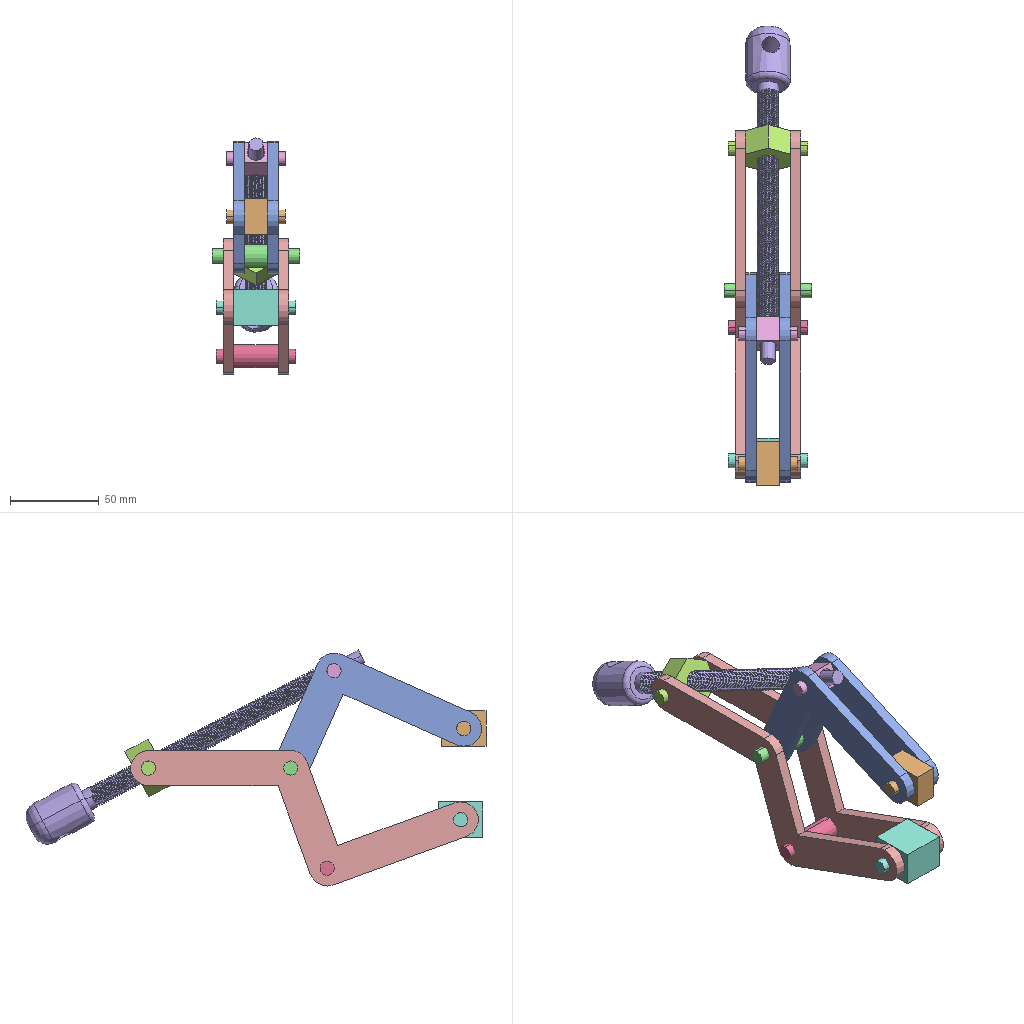Assembly | SolidWorks | 10 different items | 12 placed | box 49 x 259 x 133 mm
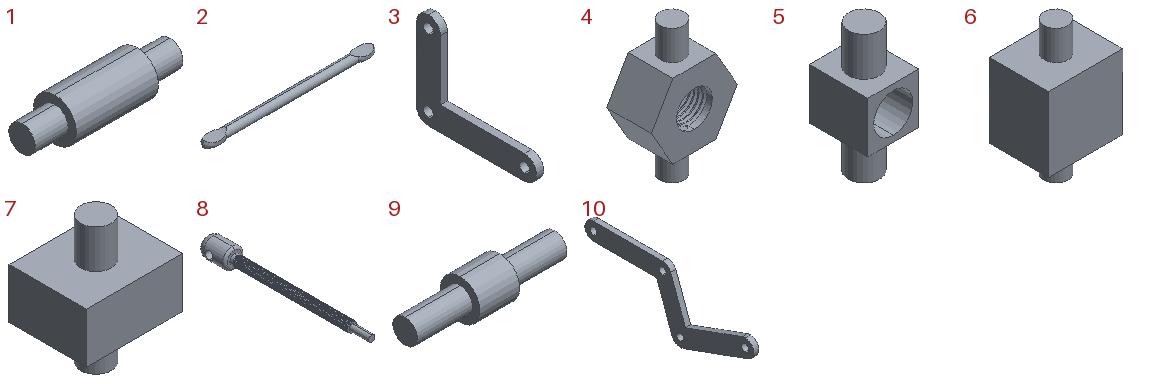Parts list (item | quantity | size | volume | features):
1 | x1 | 45 x 13 x 13 mm | 4324 mm3 | features Extrusion 1, ICE 1, MirrorPattern 1
2 | x1 | 195 x 14.893 x 10 mm | 14339 mm3 | features Extrusion 1, ICE 1, MirrorPattern 1, Revolution 1
3 | x2 | 6 x 100 x 80 mm | 17651 mm3 | features Extrusion 1
4 | x1 | 28.868 x 15 x 45 mm | 7627 mm3 | features Extrusion 1, ICE 1, MirrorPattern 1, SweepThread 1
5 | x1 | 13 x 15 x 33 mm | 2362 mm3 | features Extrusion 1, ICE 1, MirrorPattern 1
6 | x1 | 25 x 20 x 45 mm | 13505 mm3 | features Extrusion 1, ICE 1, MirrorPattern 1
7 | x1 | 25 x 20 x 33 mm | 7505 mm3 | features Extrusion 1, ICE 1, MirrorPattern 1
8 | x1 | 25 x 210 x 25 mm | 30147 mm3 | features ICE 3, Fillet 2, Extrusion 1, SweepThread 1
9 | x1 | 49 x 13 x 13 mm | 3535 mm3 | features Extrusion 1, ICE 1, MirrorPattern 1
10 | x2 | 6 x 195.697 x 76.382 mm | 26896 mm3 | features Extrusion 1
Mates (type | each side: item.copy, entity, surface, feature):
Coincident | 10.1 face plane Boss-Extrude1 | 10.2 face plane Boss-Extrude1
Concentric | 10.1 face cylinder Boss-Extrude1 | 10.2 face cylinder Boss-Extrude1
DistanceDim | 10.2 face plane Boss-Extrude1 | 10.1 face plane Boss-Extrude1
Concentric | 10.1 face cylinder Boss-Extrude1 | 3.1 face cylinder Boss-Extrude1
Coincident | 10.2 face plane Boss-Extrude1 | 3.1 face plane Boss-Extrude1
Concentric | 10.1 face cylinder Boss-Extrude1 | 3.2 face cylinder Boss-Extrude1
Coincident | 10.1 face plane Boss-Extrude1 | 3.2 face plane Boss-Extrude1
Coincident | 3.1 face plane Boss-Extrude1 | 3.2 face plane Boss-Extrude1
Concentric | 10.1 face cylinder Boss-Extrude1 | 4.1 face cylinder Boss-Extrude2
Coincident | 10.1 face plane Boss-Extrude1 | 4.1 face plane Boss-Extrude1
Concentric | 3.2 face cylinder Boss-Extrude1 | 5.1 face cylinder Boss-Extrude2
Coincident | 3.2 face plane Boss-Extrude1 | 5.1 face plane Boss-Extrude1
Concentric | 4.1 face cylinder Boss-Extrude1 | 5.1 face cylinder Boss-Extrude1
Concentric | 10.1 face cylinder Boss-Extrude1 | 6.1 face cylinder Boss-Extrude2
Coincident | 10.1 face plane Boss-Extrude1 | 6.1 face plane Boss-Extrude1
Concentric | 3.2 face cylinder Boss-Extrude1 | 7.1 face cylinder Boss-Extrude2
Coincident | 3.2 face plane Boss-Extrude1 | 7.1 face plane Boss-Extrude1
Parallel | 7.1 face plane Boss-Extrude1 | 6.1 face plane Boss-Extrude1
Concentric | 5.1 face cylinder Boss-Extrude1 | 8.1 face cylinder Boss-Extrude2
Coincident | 5.1 face plane Boss-Extrude1 | 8.1 edge
Concentric | 10.1 face cylinder Boss-Extrude1 | 9.1 face cylinder Mirror1
Coincident | 3.2 face plane Boss-Extrude1 | 9.1 face plane Boss-Extrude1
Concentric | 10.1 face cylinder Boss-Extrude1 | 1.1 face cylinder Mirror1
Coincident | 10.1 face plane Boss-Extrude1 | 1.1 face plane Boss-Extrude1